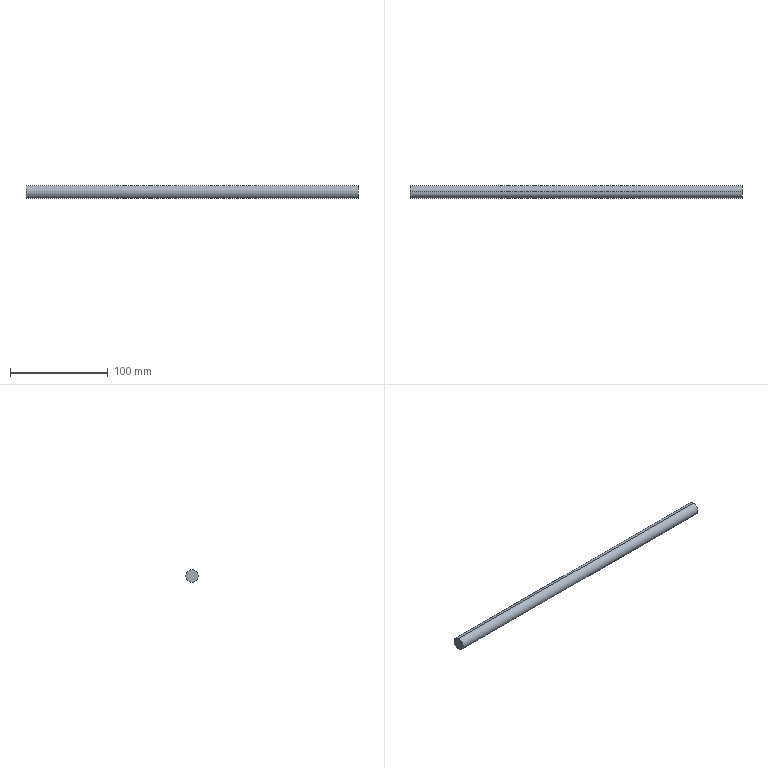Part | SolidWorks | features Extrusion 1 | 1 solid | 4 faces | box 340 x 13 x 13 mm | volume 45129 mm3 | cylinder 2 | plane 2 | commonest cylinder face diameters 13 x2
STEP:
#1=CARTESIAN_POINT('',(170.,0.,-6.5));
#2=VERTEX_POINT('',#1);
#3=CARTESIAN_POINT('',(170.,0.,6.5));
#4=VERTEX_POINT('',#3);
#5=CARTESIAN_POINT('',(170.,0.,0.));
#6=DIRECTION('',(1.,0.,0.));
#7=DIRECTION('',(0.,0.,-1.));
#8=AXIS2_PLACEMENT_3D('',#5,#6,#7);
#9=CIRCLE('',#8,6.5);
#10=EDGE_CURVE('',#2,#4,#9,.T.);
#11=ORIENTED_EDGE('',*,*,#10,.F.);
#12=CARTESIAN_POINT('',(-170.,0.,-6.5));
#13=VERTEX_POINT('',#12);
#14=CARTESIAN_POINT('',(170.,0.,-6.5));
#15=DIRECTION('',(-1.,0.,0.));
#16=VECTOR('',#15,1000.);
#17=LINE('',#14,#16);
#18=EDGE_CURVE('',#2,#13,#17,.T.);
#19=ORIENTED_EDGE('',*,*,#18,.T.);
#20=CARTESIAN_POINT('',(-170.,0.,6.5));
#21=VERTEX_POINT('',#20);
#22=CARTESIAN_POINT('',(-170.,0.,0.));
#23=DIRECTION('',(1.,0.,0.));
#24=DIRECTION('',(0.,0.,-1.));
#25=AXIS2_PLACEMENT_3D('',#22,#23,#24);
#26=CIRCLE('',#25,6.5);
#27=EDGE_CURVE('',#13,#21,#26,.T.);
#28=ORIENTED_EDGE('',*,*,#27,.T.);
#29=CARTESIAN_POINT('',(170.,0.,6.5));
#30=DIRECTION('',(-1.,0.,0.));
#31=VECTOR('',#30,1000.);
#32=LINE('',#29,#31);
#33=EDGE_CURVE('',#4,#21,#32,.T.);
#34=ORIENTED_EDGE('',*,*,#33,.F.);
#35=EDGE_LOOP('',(#11,#19,#28,#34));
#36=FACE_OUTER_BOUND('',#35,.T.);
#37=CARTESIAN_POINT('',(170.,0.,0.));
#38=DIRECTION('',(-1.,0.,0.));
#39=DIRECTION('',(0.,0.,1.));
#40=AXIS2_PLACEMENT_3D('',#37,#38,#39);
#41=CYLINDRICAL_SURFACE('',#40,6.5);
#42=ADVANCED_FACE('',(#36),#41,.T.);
#43=ORIENTED_EDGE('',*,*,#18,.F.);
#44=CARTESIAN_POINT('',(170.,0.,0.));
#45=DIRECTION('',(1.,0.,0.));
#46=DIRECTION('',(0.,0.,-1.));
#47=AXIS2_PLACEMENT_3D('',#44,#45,#46);
#48=CIRCLE('',#47,6.5);
#49=EDGE_CURVE('',#4,#2,#48,.T.);
#50=ORIENTED_EDGE('',*,*,#49,.F.);
#51=ORIENTED_EDGE('',*,*,#33,.T.);
#52=CARTESIAN_POINT('',(-170.,0.,0.));
#53=DIRECTION('',(1.,0.,0.));
#54=DIRECTION('',(0.,0.,-1.));
#55=AXIS2_PLACEMENT_3D('',#52,#53,#54);
#56=CIRCLE('',#55,6.5);
#57=EDGE_CURVE('',#21,#13,#56,.T.);
#58=ORIENTED_EDGE('',*,*,#57,.T.);
#59=EDGE_LOOP('',(#43,#50,#51,#58));
#60=FACE_OUTER_BOUND('',#59,.T.);
#61=CARTESIAN_POINT('',(170.,0.,0.));
#62=DIRECTION('',(-1.,0.,0.));
#63=DIRECTION('',(0.,0.,1.));
#64=AXIS2_PLACEMENT_3D('',#61,#62,#63);
#65=CYLINDRICAL_SURFACE('',#64,6.5);
#66=ADVANCED_FACE('',(#60),#65,.T.);
#67=ORIENTED_EDGE('',*,*,#49,.T.);
#68=ORIENTED_EDGE('',*,*,#10,.T.);
#69=EDGE_LOOP('',(#67,#68));
#70=FACE_OUTER_BOUND('',#69,.T.);
#71=CARTESIAN_POINT('',(170.,0.,0.));
#72=DIRECTION('',(1.,0.,0.));
#73=DIRECTION('',(0.,0.,-1.));
#74=AXIS2_PLACEMENT_3D('',#71,#72,#73);
#75=PLANE('',#74);
#76=ADVANCED_FACE('',(#70),#75,.T.);
#77=ORIENTED_EDGE('',*,*,#57,.F.);
#78=ORIENTED_EDGE('',*,*,#27,.F.);
#79=EDGE_LOOP('',(#77,#78));
#80=FACE_OUTER_BOUND('',#79,.T.);
#81=CARTESIAN_POINT('',(-170.,0.,0.));
#82=DIRECTION('',(1.,0.,0.));
#83=DIRECTION('',(0.,0.,-1.));
#84=AXIS2_PLACEMENT_3D('',#81,#82,#83);
#85=PLANE('',#84);
#86=ADVANCED_FACE('',(#80),#85,.F.);
#87=CLOSED_SHELL('',(#42,#66,#76,#86));
#88=MANIFOLD_SOLID_BREP('',#87);
#89=CARTESIAN_POINT('',(0.,0.,0.));
#90=DIRECTION('',(0.,0.,1.));
#91=DIRECTION('',(1.,0.,0.));
#92=AXIS2_PLACEMENT_3D('',#89,#90,#91);
#93=(LENGTH_UNIT()NAMED_UNIT(*)SI_UNIT(.MILLI.,.METRE.));
#94=UNCERTAINTY_MEASURE_WITH_UNIT(LENGTH_MEASURE(0.00001),#93,'','');
#95=(NAMED_UNIT(*)PLANE_ANGLE_UNIT()SI_UNIT($,.RADIAN.));
#96=(NAMED_UNIT(*)SI_UNIT($,.STERADIAN.)SOLID_ANGLE_UNIT());
#97=(GEOMETRIC_REPRESENTATION_CONTEXT(3)GLOBAL_UNCERTAINTY_ASSIGNED_CONTEXT((#94))GLOBAL_UNIT_ASSIGNED_CONTEXT((#93,#95,#96))REPRESENTATION_CONTEXT('',''));
#98=ADVANCED_BREP_SHAPE_REPRESENTATION('',(#88,#92),#97);